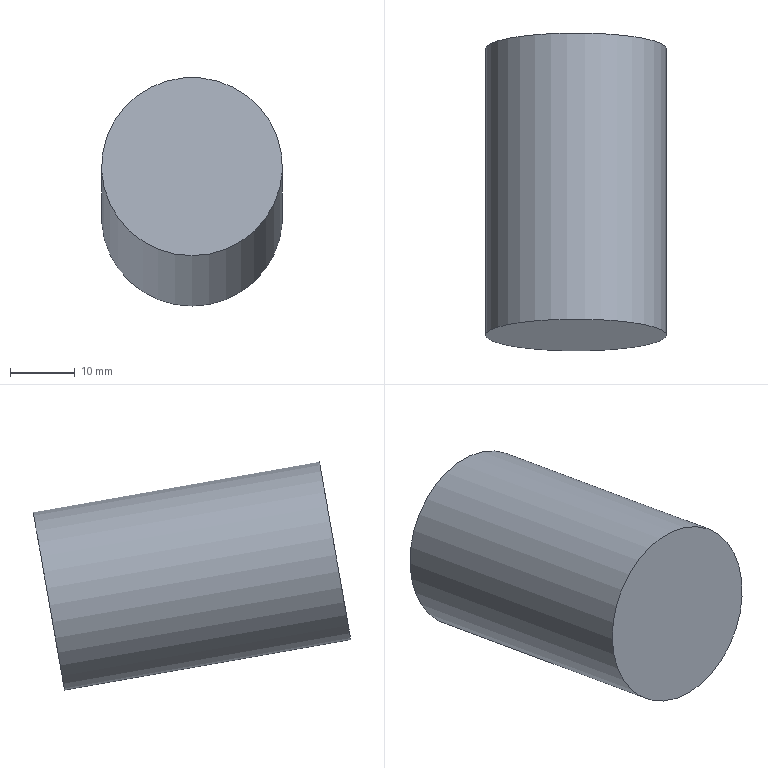Part | NX | features solid 2 | 1 solid | 3 faces | box 28 x 49.178 x 35.389 mm | volume 27709 mm3 | plane 2 | cylinder 1 | commonest cylinder face diameters 28 x1
STEP:
#1=CARTESIAN_POINT('',(653.5,-1130.005,-255.916));
#2=VERTEX_POINT('',#1);
#3=CARTESIAN_POINT('',(653.5,-1127.574,-242.128));
#4=DIRECTION('',(0.,-0.9848,0.1736));
#5=DIRECTION('',(0.,-0.1736,-0.9848));
#6=AXIS2_PLACEMENT_3D('',#3,#4,#5);
#7=CIRCLE('',#6,14.);
#8=EDGE_CURVE('',#2,#2,#7,.T.);
#9=ORIENTED_EDGE('',*,*,#8,.F.);
#10=EDGE_LOOP('',(#9));
#11=FACE_BOUND('',#10,.T.);
#12=CARTESIAN_POINT('',(653.5,-1085.689,-263.73));
#13=VERTEX_POINT('',#12);
#14=CARTESIAN_POINT('',(653.5,-1083.257,-249.942));
#15=DIRECTION('',(0.,-0.9848,0.1736));
#16=DIRECTION('',(0.,-0.1736,-0.9848));
#17=AXIS2_PLACEMENT_3D('',#14,#15,#16);
#18=CIRCLE('',#17,14.);
#19=EDGE_CURVE('',#13,#13,#18,.T.);
#20=ORIENTED_EDGE('',*,*,#19,.T.);
#21=EDGE_LOOP('',(#20));
#22=FACE_BOUND('',#21,.T.);
#23=CARTESIAN_POINT('',(653.5,-1078.826,-250.724));
#24=DIRECTION('',(0.,0.9848,-0.1736));
#25=DIRECTION('',(0.,0.1736,0.9848));
#26=AXIS2_PLACEMENT_3D('',#23,#24,#25);
#27=CYLINDRICAL_SURFACE('',#26,14.);
#28=ADVANCED_FACE('',(#11,#22),#27,.T.);
#29=ORIENTED_EDGE('',*,*,#8,.T.);
#30=EDGE_LOOP('',(#29));
#31=FACE_BOUND('',#30,.T.);
#32=CARTESIAN_POINT('',(660.,-1127.574,-242.128));
#33=DIRECTION('',(0.,-0.9848,0.1736));
#34=DIRECTION('',(0.,-0.1736,-0.9848));
#35=AXIS2_PLACEMENT_3D('',#32,#33,#34);
#36=PLANE('',#35);
#37=ADVANCED_FACE('',(#31),#36,.T.);
#38=ORIENTED_EDGE('',*,*,#19,.F.);
#39=EDGE_LOOP('',(#38));
#40=FACE_BOUND('',#39,.T.);
#41=CARTESIAN_POINT('',(660.,-1083.257,-249.942));
#42=DIRECTION('',(0.,-0.9848,0.1736));
#43=DIRECTION('',(0.,-0.1736,-0.9848));
#44=AXIS2_PLACEMENT_3D('',#41,#42,#43);
#45=PLANE('',#44);
#46=ADVANCED_FACE('',(#40),#45,.F.);
#47=CLOSED_SHELL('',(#28,#37,#46));
#48=MANIFOLD_SOLID_BREP('',#47);
#49=(LENGTH_UNIT()NAMED_UNIT(*)SI_UNIT(.MILLI.,.METRE.));
#50=UNCERTAINTY_MEASURE_WITH_UNIT(LENGTH_MEASURE(0.00001),#49,'','');
#51=(NAMED_UNIT(*)PLANE_ANGLE_UNIT()SI_UNIT($,.RADIAN.));
#52=(NAMED_UNIT(*)SI_UNIT($,.STERADIAN.)SOLID_ANGLE_UNIT());
#53=(GEOMETRIC_REPRESENTATION_CONTEXT(3)GLOBAL_UNCERTAINTY_ASSIGNED_CONTEXT((#50))GLOBAL_UNIT_ASSIGNED_CONTEXT((#49,#51,#52))REPRESENTATION_CONTEXT('',''));
#54=ADVANCED_BREP_SHAPE_REPRESENTATION('',(#48),#53);